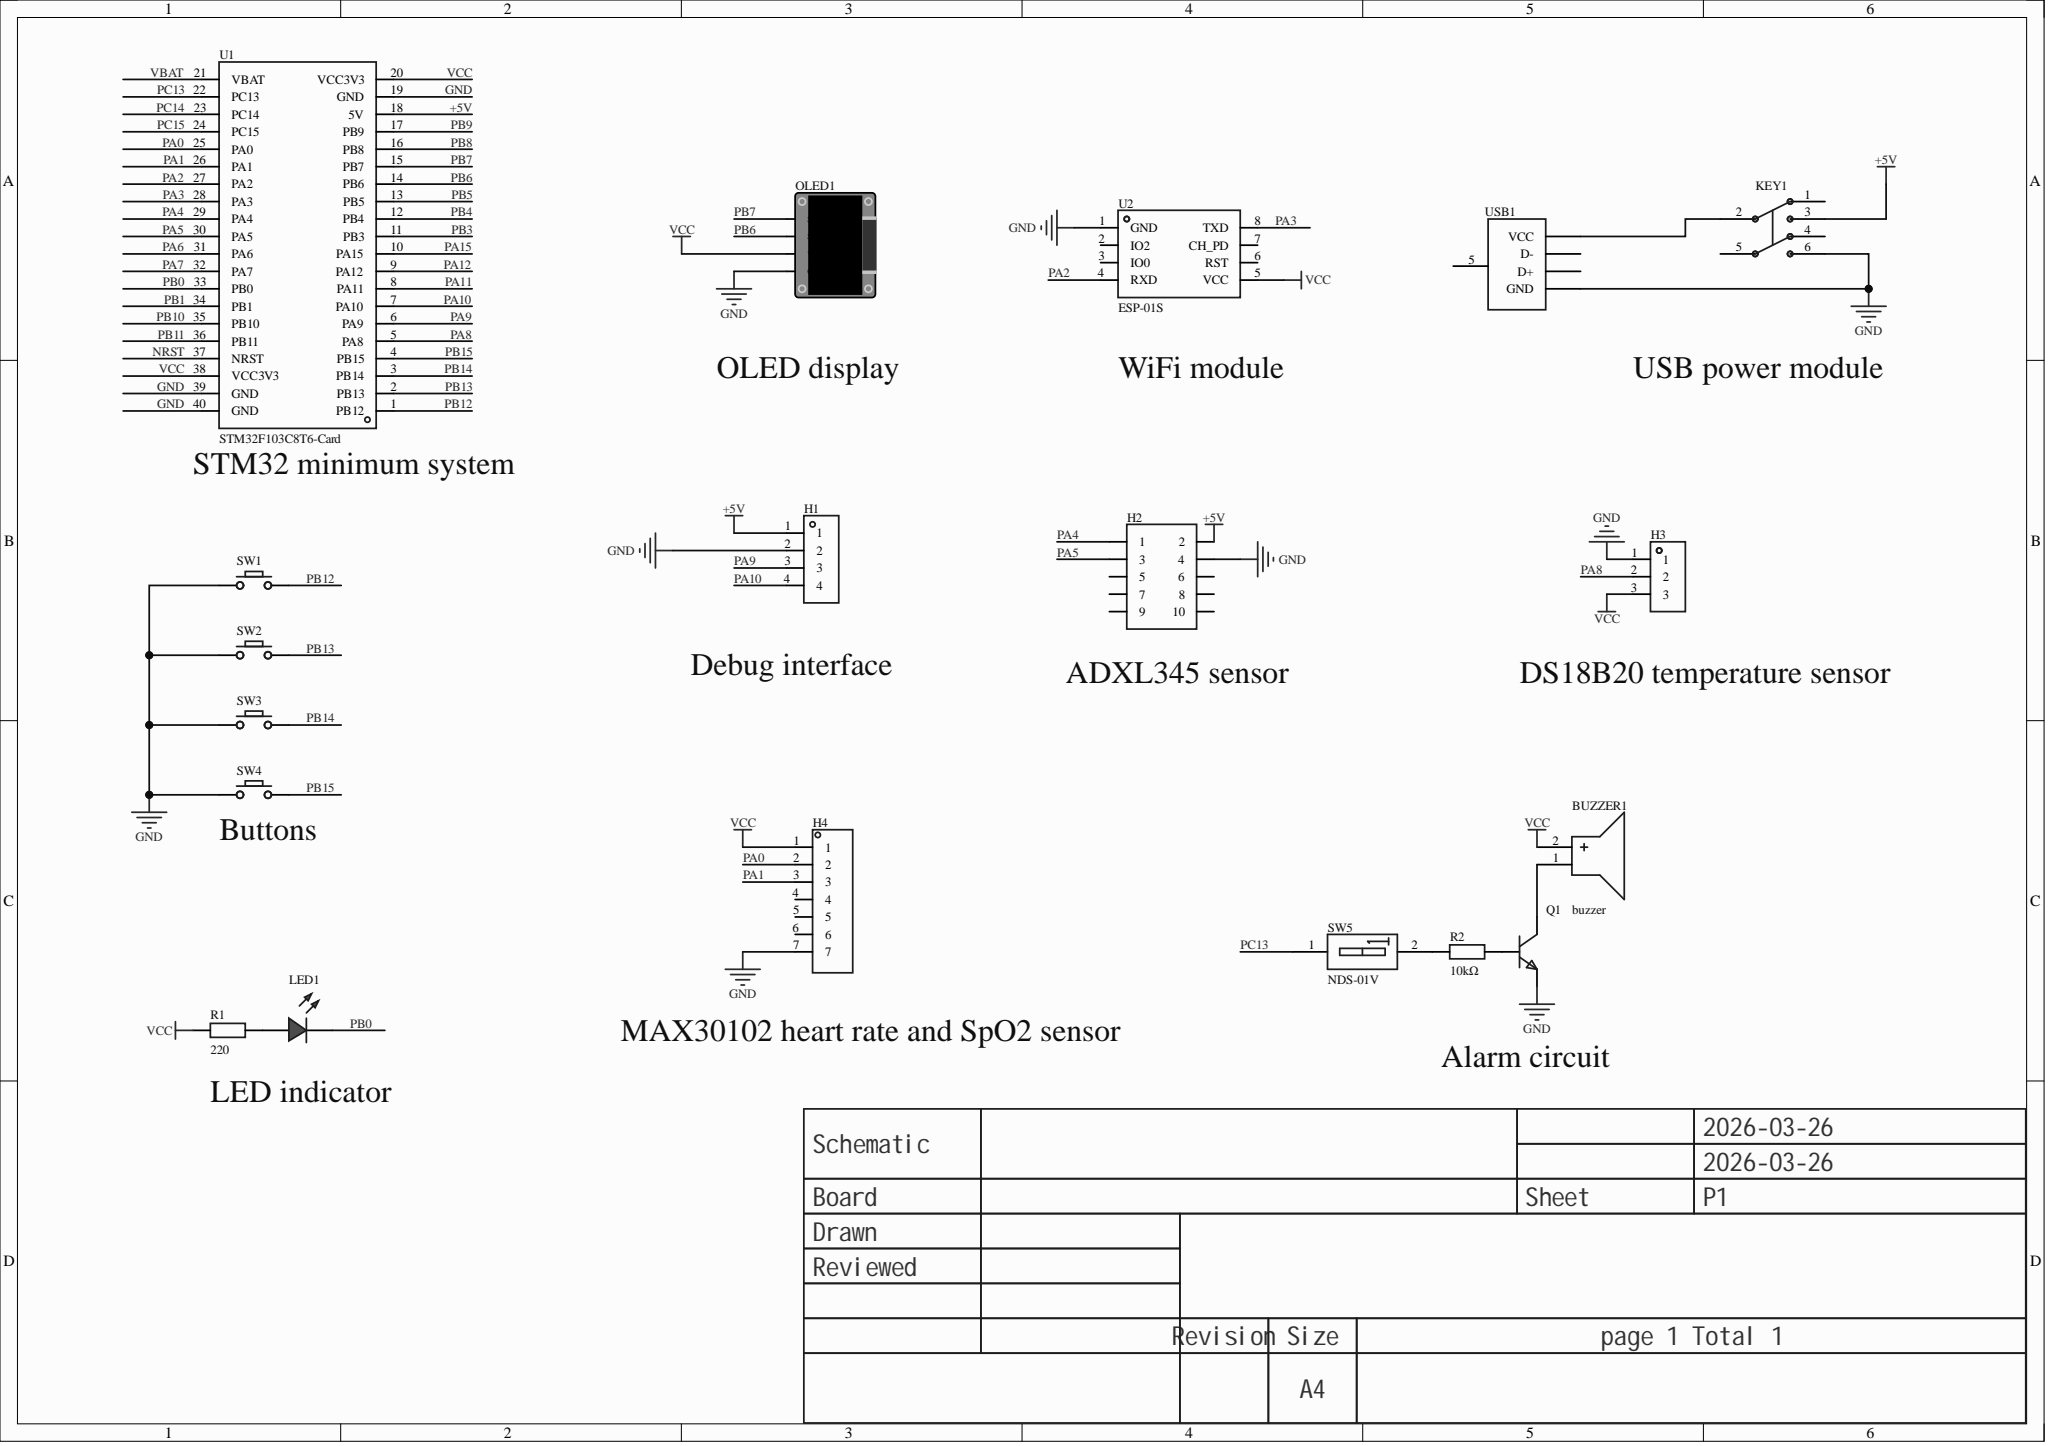Circuit board | Altium Designer | 19 parts | 25 nets
Bill of materials:
Comment,Description,Designator,Footprint,LibRef,Quantity
"buzzer","","BUZZER1","BUZ-TH_BD12.0-P6.00-D0.9-RD","buzzer","1"
"","","H1","HDR-TH_4P-P2.54-V-M","HDR-M_2.54_1x4P","1"
"","","H2","HDR-TH_10P-P2.54-V-F-R2-C5-S2.54","HDR-F_2.54_2x5","1"
"","","H3","HDR-TH_3P-P2.54-V-F","HDR-F_2.54_1x3P","1"
"","","H4","HDR-TH_7P-P2.54-V-F","HDR-F_2.54_1x7P","1"
"Non-self-locking switch 8.5×8.5 silent","6脚，8.5×8.5","KEY1","SW-TH_6P-L8.5-W8.5-P2.54","无自锁开关 8.5×8.5 无声","1"
"","","LED1","LED_TH-3mm","LED_TH-R_3mm","1"
"","","OLED1","0.96OLED_4P","0.96OLED模块_4P","1"
"","","Q1","S8050_TO_92","S8050_TO_NPN","1"
"220","","R1","Res_1/8W","Res_AXIAL-1/8W","1"
"10kΩ","","R2","Res_1/8W","Res_AXIAL-1/8W","1"
"","","SW1, SW2, SW3, SW4","Key_TH_3.5x6x4.3","Key_TH_3.5x6x4.3","4"
"NDS-01V","NDS-01V_C501305 co high-lever forward toggle","SW5","SW-TH_2P-L3.9-W9.9-P2.54-LS7.6","NDS-01V_C501305","1"
"STM32F103C8T6-Card","","U1","CONN-TH_L53.3-W22.9_STM32F103C8T6-CARD","STM32F103C8T6-Card","1"
"ESP-01S","","U2","WIFIM-TH_ESP-01S","ESP-01S_C111009","1"
"","","USB1","USB_ Type-B","USB_ Type-B","1"
Netlist (Protel format):
[
BUZZER1
BUZ-TH_BD12.0-P6.00-D0.9-RD
buzzer



]
[
H1
HDR-TH_4P-P2.54-V-M




]
[
H2
HDR-TH_10P-P2.54-V-F-R2-C5-S2.54




]
[
H3
HDR-TH_3P-P2.54-V-F




]
[
H4
HDR-TH_7P-P2.54-V-F




]
[
KEY1
SW-TH_6P-L8.5-W8.5-P2.54
Non-self-locking switch 8.5×8.5 silent



]
[
LED1
LED_TH-3mm




]
[
OLED1
0.96OLED_4P




]
[
Q1
S8050_TO_92




]
[
R1
Res_1/8W
220



]
[
R2
Res_1/8W
10kΩ



]
[
SW1
Key_TH_3.5x6x4.3




]
[
SW2
Key_TH_3.5x6x4.3




]
[
SW3
Key_TH_3.5x6x4.3




]
[
SW4
Key_TH_3.5x6x4.3




]
[
SW5
SW-TH_2P-L3.9-W9.9-P2.54-LS7.6
NDS-01V



]
[
U1
CONN-TH_L53.3-W22.9_STM32F103C8T6-CARD
STM32F103C8T6-Card



]
[
U2
WIFIM-TH_ESP-01S
ESP-01S



]
[
USB1
USB_ Type-B




]
(
VCC
BUZZER1-2
H3-3
H4-1
OLED1-2
R1-1
U1-20
U1-38
U2-5
)
(
PC13
SW5-1
U1-22
)
(
PB15
SW4-B
U1-4
)
(
PB14
SW3-B
U1-3
)
(
PB13
SW2-B
U1-2
)
(
PB12
SW1-B
U1-1
)
(
PB7
OLED1-4
U1-15
)
(
PB6
OLED1-3
U1-14
)
(
PB0
LED1-2
U1-33
)
(
PA10
H1-4
U1-7
)
(
PA9
H1-3
U1-6
)
(
PA8
H3-2
U1-5
)
(
PA5
H2-3
U1-30
)
(
PA4
H2-1
U1-29
)
(
PA3
U1-28
U2-8
)
(
PA2
U1-27
U2-4
)
(
PA1
H4-3
U1-26
)
(
PA0
H4-2
U1-25
)
(
NetR2_1
R2-1
SW5-2
)
(
NetQ1_2
Q1-2
R2-2
)
(
NetLED1_1
LED1-1
R1-2
)
(
NetKEY1_2
KEY1-2
USB1-1
)
(
NetBUZZER1_1
BUZZER1-1
Q1-3
)
(
GND
H1-2
H2-4
H3-1
H4-7
KEY1-6
OLED1-1
Q1-1
SW1-A
SW2-A
SW3-A
SW4-A
U1-19
U1-39
U1-40
U2-1
USB1-4
)
(
+5V
H1-1
H2-2
KEY1-3
U1-18
)